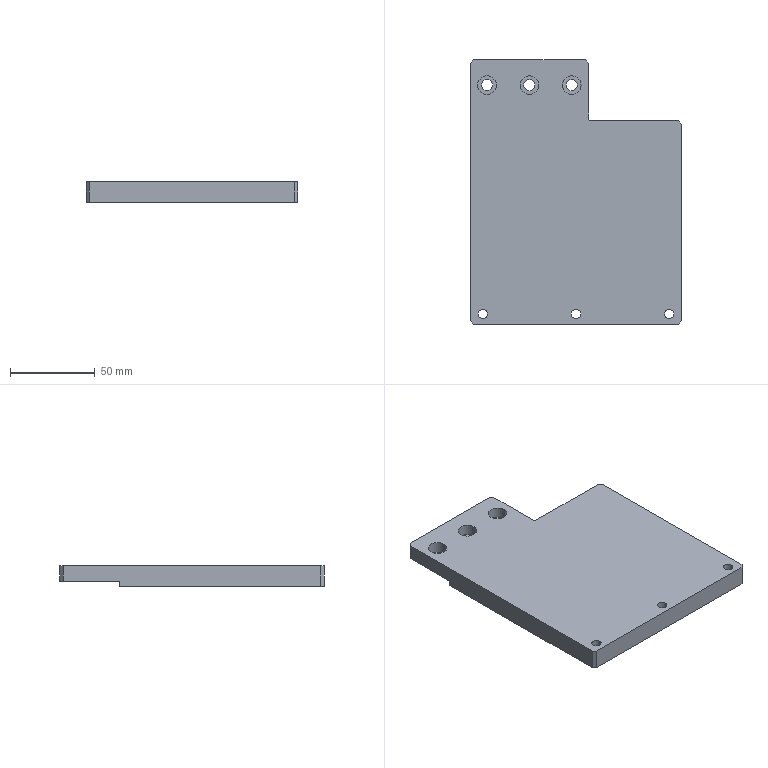Part | SolidWorks | features HoleWzd 2, ICE 2, Chamfer 1, Extrusion 1, Fillet 1 | 1 solid | 46 faces | box 125 x 156 x 12 mm | volume 198828 mm3 | cylinder 25 | plane 21 | commonest cylinder face diameters 5.5 x6 6.6 x6 10 x6 11 x6 2 x1
STEP:
#1=CARTESIAN_POINT('',(-8.,63.,5.2));
#2=VERTEX_POINT('',#1);
#3=CARTESIAN_POINT('',(3.,63.,5.2));
#4=VERTEX_POINT('',#3);
#5=CARTESIAN_POINT('',(-2.5,63.,5.2));
#6=DIRECTION('',(0.,0.,1.));
#7=DIRECTION('',(1.,0.,0.));
#8=AXIS2_PLACEMENT_3D('',#5,#6,#7);
#9=CIRCLE('',#8,5.5);
#10=EDGE_CURVE('',#2,#4,#9,.T.);
#11=ORIENTED_EDGE('',*,*,#10,.F.);
#12=CARTESIAN_POINT('',(-8.,63.,12.));
#13=VERTEX_POINT('',#12);
#14=CARTESIAN_POINT('',(-8.,63.,12.));
#15=DIRECTION('',(0.,0.,1.));
#16=VECTOR('',#15,1000.);
#17=LINE('',#14,#16);
#18=EDGE_CURVE('',#2,#13,#17,.T.);
#19=ORIENTED_EDGE('',*,*,#18,.T.);
#20=CARTESIAN_POINT('',(3.,63.,12.));
#21=VERTEX_POINT('',#20);
#22=CARTESIAN_POINT('',(-2.5,63.,12.));
#23=DIRECTION('',(0.,0.,1.));
#24=DIRECTION('',(1.,0.,0.));
#25=AXIS2_PLACEMENT_3D('',#22,#23,#24);
#26=CIRCLE('',#25,5.5);
#27=EDGE_CURVE('',#13,#21,#26,.T.);
#28=ORIENTED_EDGE('',*,*,#27,.T.);
#29=CARTESIAN_POINT('',(3.,63.,12.));
#30=DIRECTION('',(0.,0.,1.));
#31=VECTOR('',#30,1000.);
#32=LINE('',#29,#31);
#33=EDGE_CURVE('',#4,#21,#32,.T.);
#34=ORIENTED_EDGE('',*,*,#33,.F.);
#35=EDGE_LOOP('',(#11,#19,#28,#34));
#36=FACE_OUTER_BOUND('',#35,.T.);
#37=CARTESIAN_POINT('',(-2.5,63.,12.));
#38=DIRECTION('',(0.,0.,1.));
#39=DIRECTION('',(1.,0.,0.));
#40=AXIS2_PLACEMENT_3D('',#37,#38,#39);
#41=CYLINDRICAL_SURFACE('',#40,5.5);
#42=ADVANCED_FACE('',(#36),#41,.F.);
#43=CARTESIAN_POINT('',(-5.8,63.,3.));
#44=VERTEX_POINT('',#43);
#45=CARTESIAN_POINT('',(0.8,63.,3.));
#46=VERTEX_POINT('',#45);
#47=CARTESIAN_POINT('',(-2.5,63.,3.));
#48=DIRECTION('',(0.,0.,1.));
#49=DIRECTION('',(1.,0.,0.));
#50=AXIS2_PLACEMENT_3D('',#47,#48,#49);
#51=CIRCLE('',#50,3.3);
#52=EDGE_CURVE('',#44,#46,#51,.T.);
#53=ORIENTED_EDGE('',*,*,#52,.F.);
#54=CARTESIAN_POINT('',(-5.8,63.,5.2));
#55=VERTEX_POINT('',#54);
#56=CARTESIAN_POINT('',(-5.8,63.,12.));
#57=DIRECTION('',(0.,0.,1.));
#58=VECTOR('',#57,1000.);
#59=LINE('',#56,#58);
#60=EDGE_CURVE('',#44,#55,#59,.T.);
#61=ORIENTED_EDGE('',*,*,#60,.T.);
#62=CARTESIAN_POINT('',(0.8,63.,5.2));
#63=VERTEX_POINT('',#62);
#64=CARTESIAN_POINT('',(-2.5,63.,5.2));
#65=DIRECTION('',(0.,0.,1.));
#66=DIRECTION('',(1.,0.,0.));
#67=AXIS2_PLACEMENT_3D('',#64,#65,#66);
#68=CIRCLE('',#67,3.3);
#69=EDGE_CURVE('',#55,#63,#68,.T.);
#70=ORIENTED_EDGE('',*,*,#69,.T.);
#71=CARTESIAN_POINT('',(0.8,63.,12.));
#72=DIRECTION('',(0.,0.,1.));
#73=VECTOR('',#72,1000.);
#74=LINE('',#71,#73);
#75=EDGE_CURVE('',#46,#63,#74,.T.);
#76=ORIENTED_EDGE('',*,*,#75,.F.);
#77=EDGE_LOOP('',(#53,#61,#70,#76));
#78=FACE_OUTER_BOUND('',#77,.T.);
#79=CARTESIAN_POINT('',(-2.5,63.,12.));
#80=DIRECTION('',(0.,0.,1.));
#81=DIRECTION('',(1.,0.,0.));
#82=AXIS2_PLACEMENT_3D('',#79,#80,#81);
#83=CYLINDRICAL_SURFACE('',#82,3.3);
#84=ADVANCED_FACE('',(#78),#83,.F.);
#85=CARTESIAN_POINT('',(-33.,63.,5.2));
#86=VERTEX_POINT('',#85);
#87=CARTESIAN_POINT('',(-22.,63.,5.2));
#88=VERTEX_POINT('',#87);
#89=CARTESIAN_POINT('',(-27.5,63.,5.2));
#90=DIRECTION('',(0.,0.,1.));
#91=DIRECTION('',(1.,0.,0.));
#92=AXIS2_PLACEMENT_3D('',#89,#90,#91);
#93=CIRCLE('',#92,5.5);
#94=EDGE_CURVE('',#86,#88,#93,.T.);
#95=ORIENTED_EDGE('',*,*,#94,.F.);
#96=CARTESIAN_POINT('',(-33.,63.,12.));
#97=VERTEX_POINT('',#96);
#98=CARTESIAN_POINT('',(-33.,63.,12.));
#99=DIRECTION('',(0.,0.,1.));
#100=VECTOR('',#99,1000.);
#101=LINE('',#98,#100);
#102=EDGE_CURVE('',#86,#97,#101,.T.);
#103=ORIENTED_EDGE('',*,*,#102,.T.);
#104=CARTESIAN_POINT('',(-22.,63.,12.));
#105=VERTEX_POINT('',#104);
#106=CARTESIAN_POINT('',(-27.5,63.,12.));
#107=DIRECTION('',(0.,0.,1.));
#108=DIRECTION('',(1.,0.,0.));
#109=AXIS2_PLACEMENT_3D('',#106,#107,#108);
#110=CIRCLE('',#109,5.5);
#111=EDGE_CURVE('',#97,#105,#110,.T.);
#112=ORIENTED_EDGE('',*,*,#111,.T.);
#113=CARTESIAN_POINT('',(-22.,63.,12.));
#114=DIRECTION('',(0.,0.,1.));
#115=VECTOR('',#114,1000.);
#116=LINE('',#113,#115);
#117=EDGE_CURVE('',#88,#105,#116,.T.);
#118=ORIENTED_EDGE('',*,*,#117,.F.);
#119=EDGE_LOOP('',(#95,#103,#112,#118));
#120=FACE_OUTER_BOUND('',#119,.T.);
#121=CARTESIAN_POINT('',(-27.5,63.,12.));
#122=DIRECTION('',(0.,0.,1.));
#123=DIRECTION('',(1.,0.,0.));
#124=AXIS2_PLACEMENT_3D('',#121,#122,#123);
#125=CYLINDRICAL_SURFACE('',#124,5.5);
#126=ADVANCED_FACE('',(#120),#125,.F.);
#127=CARTESIAN_POINT('',(-30.8,63.,3.));
#128=VERTEX_POINT('',#127);
#129=CARTESIAN_POINT('',(-24.2,63.,3.));
#130=VERTEX_POINT('',#129);
#131=CARTESIAN_POINT('',(-27.5,63.,3.));
#132=DIRECTION('',(0.,0.,1.));
#133=DIRECTION('',(1.,0.,0.));
#134=AXIS2_PLACEMENT_3D('',#131,#132,#133);
#135=CIRCLE('',#134,3.3);
#136=EDGE_CURVE('',#128,#130,#135,.T.);
#137=ORIENTED_EDGE('',*,*,#136,.F.);
#138=CARTESIAN_POINT('',(-30.8,63.,5.2));
#139=VERTEX_POINT('',#138);
#140=CARTESIAN_POINT('',(-30.8,63.,12.));
#141=DIRECTION('',(0.,0.,1.));
#142=VECTOR('',#141,1000.);
#143=LINE('',#140,#142);
#144=EDGE_CURVE('',#128,#139,#143,.T.);
#145=ORIENTED_EDGE('',*,*,#144,.T.);
#146=CARTESIAN_POINT('',(-24.2,63.,5.2));
#147=VERTEX_POINT('',#146);
#148=CARTESIAN_POINT('',(-27.5,63.,5.2));
#149=DIRECTION('',(0.,0.,1.));
#150=DIRECTION('',(1.,0.,0.));
#151=AXIS2_PLACEMENT_3D('',#148,#149,#150);
#152=CIRCLE('',#151,3.3);
#153=EDGE_CURVE('',#139,#147,#152,.T.);
#154=ORIENTED_EDGE('',*,*,#153,.T.);
#155=CARTESIAN_POINT('',(-24.2,63.,12.));
#156=DIRECTION('',(0.,0.,1.));
#157=VECTOR('',#156,1000.);
#158=LINE('',#155,#157);
#159=EDGE_CURVE('',#130,#147,#158,.T.);
#160=ORIENTED_EDGE('',*,*,#159,.F.);
#161=EDGE_LOOP('',(#137,#145,#154,#160));
#162=FACE_OUTER_BOUND('',#161,.T.);
#163=CARTESIAN_POINT('',(-27.5,63.,12.));
#164=DIRECTION('',(0.,0.,1.));
#165=DIRECTION('',(1.,0.,0.));
#166=AXIS2_PLACEMENT_3D('',#163,#164,#165);
#167=CYLINDRICAL_SURFACE('',#166,3.3);
#168=ADVANCED_FACE('',(#162),#167,.F.);
#169=CARTESIAN_POINT('',(-58.,63.,5.2));
#170=VERTEX_POINT('',#169);
#171=CARTESIAN_POINT('',(-47.,63.,5.2));
#172=VERTEX_POINT('',#171);
#173=CARTESIAN_POINT('',(-52.5,63.,5.2));
#174=DIRECTION('',(0.,0.,1.));
#175=DIRECTION('',(1.,0.,0.));
#176=AXIS2_PLACEMENT_3D('',#173,#174,#175);
#177=CIRCLE('',#176,5.5);
#178=EDGE_CURVE('',#170,#172,#177,.T.);
#179=ORIENTED_EDGE('',*,*,#178,.F.);
#180=CARTESIAN_POINT('',(-58.,63.,12.));
#181=VERTEX_POINT('',#180);
#182=CARTESIAN_POINT('',(-58.,63.,12.));
#183=DIRECTION('',(0.,0.,1.));
#184=VECTOR('',#183,1000.);
#185=LINE('',#182,#184);
#186=EDGE_CURVE('',#170,#181,#185,.T.);
#187=ORIENTED_EDGE('',*,*,#186,.T.);
#188=CARTESIAN_POINT('',(-47.,63.,12.));
#189=VERTEX_POINT('',#188);
#190=CARTESIAN_POINT('',(-52.5,63.,12.));
#191=DIRECTION('',(0.,0.,1.));
#192=DIRECTION('',(1.,0.,0.));
#193=AXIS2_PLACEMENT_3D('',#190,#191,#192);
#194=CIRCLE('',#193,5.5);
#195=EDGE_CURVE('',#181,#189,#194,.T.);
#196=ORIENTED_EDGE('',*,*,#195,.T.);
#197=CARTESIAN_POINT('',(-47.,63.,12.));
#198=DIRECTION('',(0.,0.,1.));
#199=VECTOR('',#198,1000.);
#200=LINE('',#197,#199);
#201=EDGE_CURVE('',#172,#189,#200,.T.);
#202=ORIENTED_EDGE('',*,*,#201,.F.);
#203=EDGE_LOOP('',(#179,#187,#196,#202));
#204=FACE_OUTER_BOUND('',#203,.T.);
#205=CARTESIAN_POINT('',(-52.5,63.,12.));
#206=DIRECTION('',(0.,0.,1.));
#207=DIRECTION('',(1.,0.,0.));
#208=AXIS2_PLACEMENT_3D('',#205,#206,#207);
#209=CYLINDRICAL_SURFACE('',#208,5.5);
#210=ADVANCED_FACE('',(#204),#209,.F.);
#211=CARTESIAN_POINT('',(-55.8,63.,3.));
#212=VERTEX_POINT('',#211);
#213=CARTESIAN_POINT('',(-49.2,63.,3.));
#214=VERTEX_POINT('',#213);
#215=CARTESIAN_POINT('',(-52.5,63.,3.));
#216=DIRECTION('',(0.,0.,1.));
#217=DIRECTION('',(1.,0.,0.));
#218=AXIS2_PLACEMENT_3D('',#215,#216,#217);
#219=CIRCLE('',#218,3.3);
#220=EDGE_CURVE('',#212,#214,#219,.T.);
#221=ORIENTED_EDGE('',*,*,#220,.F.);
#222=CARTESIAN_POINT('',(-55.8,63.,5.2));
#223=VERTEX_POINT('',#222);
#224=CARTESIAN_POINT('',(-55.8,63.,12.));
#225=DIRECTION('',(0.,0.,1.));
#226=VECTOR('',#225,1000.);
#227=LINE('',#224,#226);
#228=EDGE_CURVE('',#212,#223,#227,.T.);
#229=ORIENTED_EDGE('',*,*,#228,.T.);
#230=CARTESIAN_POINT('',(-49.2,63.,5.2));
#231=VERTEX_POINT('',#230);
#232=CARTESIAN_POINT('',(-52.5,63.,5.2));
#233=DIRECTION('',(0.,0.,1.));
#234=DIRECTION('',(1.,0.,0.));
#235=AXIS2_PLACEMENT_3D('',#232,#233,#234);
#236=CIRCLE('',#235,3.3);
#237=EDGE_CURVE('',#223,#231,#236,.T.);
#238=ORIENTED_EDGE('',*,*,#237,.T.);
#239=CARTESIAN_POINT('',(-49.2,63.,12.));
#240=DIRECTION('',(0.,0.,1.));
#241=VECTOR('',#240,1000.);
#242=LINE('',#239,#241);
#243=EDGE_CURVE('',#214,#231,#242,.T.);
#244=ORIENTED_EDGE('',*,*,#243,.F.);
#245=EDGE_LOOP('',(#221,#229,#238,#244));
#246=FACE_OUTER_BOUND('',#245,.T.);
#247=CARTESIAN_POINT('',(-52.5,63.,12.));
#248=DIRECTION('',(0.,0.,1.));
#249=DIRECTION('',(1.,0.,0.));
#250=AXIS2_PLACEMENT_3D('',#247,#248,#249);
#251=CYLINDRICAL_SURFACE('',#250,3.3);
#252=ADVANCED_FACE('',(#246),#251,.F.);
#253=CARTESIAN_POINT('',(60.,-72.,5.7));
#254=VERTEX_POINT('',#253);
#255=CARTESIAN_POINT('',(50.,-72.,5.7));
#256=VERTEX_POINT('',#255);
#257=CARTESIAN_POINT('',(55.,-72.,5.7));
#258=DIRECTION('',(0.,0.,-1.));
#259=DIRECTION('',(-1.,0.,0.));
#260=AXIS2_PLACEMENT_3D('',#257,#258,#259);
#261=CIRCLE('',#260,5.);
#262=EDGE_CURVE('',#254,#256,#261,.T.);
#263=ORIENTED_EDGE('',*,*,#262,.F.);
#264=CARTESIAN_POINT('',(60.,-72.,0.));
#265=VERTEX_POINT('',#264);
#266=CARTESIAN_POINT('',(60.,-72.,0.));
#267=DIRECTION('',(0.,0.,-1.));
#268=VECTOR('',#267,1000.);
#269=LINE('',#266,#268);
#270=EDGE_CURVE('',#254,#265,#269,.T.);
#271=ORIENTED_EDGE('',*,*,#270,.T.);
#272=CARTESIAN_POINT('',(50.,-72.,0.));
#273=VERTEX_POINT('',#272);
#274=CARTESIAN_POINT('',(55.,-72.,0.));
#275=DIRECTION('',(0.,0.,-1.));
#276=DIRECTION('',(-1.,0.,0.));
#277=AXIS2_PLACEMENT_3D('',#274,#275,#276);
#278=CIRCLE('',#277,5.);
#279=EDGE_CURVE('',#265,#273,#278,.T.);
#280=ORIENTED_EDGE('',*,*,#279,.T.);
#281=CARTESIAN_POINT('',(50.,-72.,0.));
#282=DIRECTION('',(0.,0.,-1.));
#283=VECTOR('',#282,1000.);
#284=LINE('',#281,#283);
#285=EDGE_CURVE('',#256,#273,#284,.T.);
#286=ORIENTED_EDGE('',*,*,#285,.F.);
#287=EDGE_LOOP('',(#263,#271,#280,#286));
#288=FACE_OUTER_BOUND('',#287,.T.);
#289=CARTESIAN_POINT('',(55.,-72.,0.));
#290=DIRECTION('',(0.,0.,-1.));
#291=DIRECTION('',(-1.,0.,0.));
#292=AXIS2_PLACEMENT_3D('',#289,#290,#291);
#293=CYLINDRICAL_SURFACE('',#292,5.);
#294=ADVANCED_FACE('',(#288),#293,.F.);
#295=CARTESIAN_POINT('',(57.75,-72.,12.));
#296=VERTEX_POINT('',#295);
#297=CARTESIAN_POINT('',(52.25,-72.,12.));
#298=VERTEX_POINT('',#297);
#299=CARTESIAN_POINT('',(55.,-72.,12.));
#300=DIRECTION('',(0.,0.,-1.));
#301=DIRECTION('',(-1.,0.,0.));
#302=AXIS2_PLACEMENT_3D('',#299,#300,#301);
#303=CIRCLE('',#302,2.75);
#304=EDGE_CURVE('',#296,#298,#303,.T.);
#305=ORIENTED_EDGE('',*,*,#304,.F.);
#306=CARTESIAN_POINT('',(57.75,-72.,5.7));
#307=VERTEX_POINT('',#306);
#308=CARTESIAN_POINT('',(57.75,-72.,0.));
#309=DIRECTION('',(0.,0.,-1.));
#310=VECTOR('',#309,1000.);
#311=LINE('',#308,#310);
#312=EDGE_CURVE('',#296,#307,#311,.T.);
#313=ORIENTED_EDGE('',*,*,#312,.T.);
#314=CARTESIAN_POINT('',(52.25,-72.,5.7));
#315=VERTEX_POINT('',#314);
#316=CARTESIAN_POINT('',(55.,-72.,5.7));
#317=DIRECTION('',(0.,0.,-1.));
#318=DIRECTION('',(-1.,0.,0.));
#319=AXIS2_PLACEMENT_3D('',#316,#317,#318);
#320=CIRCLE('',#319,2.75);
#321=EDGE_CURVE('',#307,#315,#320,.T.);
#322=ORIENTED_EDGE('',*,*,#321,.T.);
#323=CARTESIAN_POINT('',(52.25,-72.,0.));
#324=DIRECTION('',(0.,0.,-1.));
#325=VECTOR('',#324,1000.);
#326=LINE('',#323,#325);
#327=EDGE_CURVE('',#298,#315,#326,.T.);
#328=ORIENTED_EDGE('',*,*,#327,.F.);
#329=EDGE_LOOP('',(#305,#313,#322,#328));
#330=FACE_OUTER_BOUND('',#329,.T.);
#331=CARTESIAN_POINT('',(55.,-72.,0.));
#332=DIRECTION('',(0.,0.,-1.));
#333=DIRECTION('',(-1.,0.,0.));
#334=AXIS2_PLACEMENT_3D('',#331,#332,#333);
#335=CYLINDRICAL_SURFACE('',#334,2.75);
#336=ADVANCED_FACE('',(#330),#335,.F.);
#337=CARTESIAN_POINT('',(5.,-72.,5.7));
#338=VERTEX_POINT('',#337);
#339=CARTESIAN_POINT('',(-5.,-72.,5.7));
#340=VERTEX_POINT('',#339);
#341=CARTESIAN_POINT('',(0.,-72.,5.7));
#342=DIRECTION('',(0.,0.,-1.));
#343=DIRECTION('',(-1.,0.,0.));
#344=AXIS2_PLACEMENT_3D('',#341,#342,#343);
#345=CIRCLE('',#344,5.);
#346=EDGE_CURVE('',#338,#340,#345,.T.);
#347=ORIENTED_EDGE('',*,*,#346,.F.);
#348=CARTESIAN_POINT('',(5.,-72.,0.));
#349=VERTEX_POINT('',#348);
#350=CARTESIAN_POINT('',(5.,-72.,0.));
#351=DIRECTION('',(0.,0.,-1.));
#352=VECTOR('',#351,1000.);
#353=LINE('',#350,#352);
#354=EDGE_CURVE('',#338,#349,#353,.T.);
#355=ORIENTED_EDGE('',*,*,#354,.T.);
#356=CARTESIAN_POINT('',(-5.,-72.,0.));
#357=VERTEX_POINT('',#356);
#358=CARTESIAN_POINT('',(0.,-72.,0.));
#359=DIRECTION('',(0.,0.,-1.));
#360=DIRECTION('',(-1.,0.,0.));
#361=AXIS2_PLACEMENT_3D('',#358,#359,#360);
#362=CIRCLE('',#361,5.);
#363=EDGE_CURVE('',#349,#357,#362,.T.);
#364=ORIENTED_EDGE('',*,*,#363,.T.);
#365=CARTESIAN_POINT('',(-5.,-72.,0.));
#366=DIRECTION('',(0.,0.,-1.));
#367=VECTOR('',#366,1000.);
#368=LINE('',#365,#367);
#369=EDGE_CURVE('',#340,#357,#368,.T.);
#370=ORIENTED_EDGE('',*,*,#369,.F.);
#371=EDGE_LOOP('',(#347,#355,#364,#370));
#372=FACE_OUTER_BOUND('',#371,.T.);
#373=CARTESIAN_POINT('',(0.,-72.,0.));
#374=DIRECTION('',(0.,0.,-1.));
#375=DIRECTION('',(-1.,0.,0.));
#376=AXIS2_PLACEMENT_3D('',#373,#374,#375);
#377=CYLINDRICAL_SURFACE('',#376,5.);
#378=ADVANCED_FACE('',(#372),#377,.F.);
#379=CARTESIAN_POINT('',(2.75,-72.,12.));
#380=VERTEX_POINT('',#379);
#381=CARTESIAN_POINT('',(-2.75,-72.,12.));
#382=VERTEX_POINT('',#381);
#383=CARTESIAN_POINT('',(0.,-72.,12.));
#384=DIRECTION('',(0.,0.,-1.));
#385=DIRECTION('',(-1.,0.,0.));
#386=AXIS2_PLACEMENT_3D('',#383,#384,#385);
#387=CIRCLE('',#386,2.75);
#388=EDGE_CURVE('',#380,#382,#387,.T.);
#389=ORIENTED_EDGE('',*,*,#388,.F.);
#390=CARTESIAN_POINT('',(2.75,-72.,5.7));
#391=VERTEX_POINT('',#390);
#392=CARTESIAN_POINT('',(2.75,-72.,0.));
#393=DIRECTION('',(0.,0.,-1.));
#394=VECTOR('',#393,1000.);
#395=LINE('',#392,#394);
#396=EDGE_CURVE('',#380,#391,#395,.T.);
#397=ORIENTED_EDGE('',*,*,#396,.T.);
#398=CARTESIAN_POINT('',(-2.75,-72.,5.7));
#399=VERTEX_POINT('',#398);
#400=CARTESIAN_POINT('',(0.,-72.,5.7));
#401=DIRECTION('',(0.,0.,-1.));
#402=DIRECTION('',(-1.,0.,0.));
#403=AXIS2_PLACEMENT_3D('',#400,#401,#402);
#404=CIRCLE('',#403,2.75);
#405=EDGE_CURVE('',#391,#399,#404,.T.);
#406=ORIENTED_EDGE('',*,*,#405,.T.);
#407=CARTESIAN_POINT('',(-2.75,-72.,0.));
#408=DIRECTION('',(0.,0.,-1.));
#409=VECTOR('',#408,1000.);
#410=LINE('',#407,#409);
#411=EDGE_CURVE('',#382,#399,#410,.T.);
#412=ORIENTED_EDGE('',*,*,#411,.F.);
#413=EDGE_LOOP('',(#389,#397,#406,#412));
#414=FACE_OUTER_BOUND('',#413,.T.);
#415=CARTESIAN_POINT('',(0.,-72.,0.));
#416=DIRECTION('',(0.,0.,-1.));
#417=DIRECTION('',(-1.,0.,0.));
#418=AXIS2_PLACEMENT_3D('',#415,#416,#417);
#419=CYLINDRICAL_SURFACE('',#418,2.75);
#420=ADVANCED_FACE('',(#414),#419,.F.);
#421=CARTESIAN_POINT('',(-50.,-72.,5.7));
#422=VERTEX_POINT('',#421);
#423=CARTESIAN_POINT('',(-60.,-72.,5.7));
#424=VERTEX_POINT('',#423);
#425=CARTESIAN_POINT('',(-55.,-72.,5.7));
#426=DIRECTION('',(0.,0.,-1.));
#427=DIRECTION('',(-1.,0.,0.));
#428=AXIS2_PLACEMENT_3D('',#425,#426,#427);
#429=CIRCLE('',#428,5.);
#430=EDGE_CURVE('',#422,#424,#429,.T.);
#431=ORIENTED_EDGE('',*,*,#430,.F.);
#432=CARTESIAN_POINT('',(-50.,-72.,0.));
#433=VERTEX_POINT('',#432);
#434=CARTESIAN_POINT('',(-50.,-72.,0.));
#435=DIRECTION('',(0.,0.,-1.));
#436=VECTOR('',#435,1000.);
#437=LINE('',#434,#436);
#438=EDGE_CURVE('',#422,#433,#437,.T.);
#439=ORIENTED_EDGE('',*,*,#438,.T.);
#440=CARTESIAN_POINT('',(-60.,-72.,0.));
#441=VERTEX_POINT('',#440);
#442=CARTESIAN_POINT('',(-55.,-72.,0.));
#443=DIRECTION('',(0.,0.,-1.));
#444=DIRECTION('',(-1.,0.,0.));
#445=AXIS2_PLACEMENT_3D('',#442,#443,#444);
#446=CIRCLE('',#445,5.);
#447=EDGE_CURVE('',#433,#441,#446,.T.);
#448=ORIENTED_EDGE('',*,*,#447,.T.);
#449=CARTESIAN_POINT('',(-60.,-72.,0.));
#450=DIRECTION('',(0.,0.,-1.));
#451=VECTOR('',#450,1000.);
#452=LINE('',#449,#451);
#453=EDGE_CURVE('',#424,#441,#452,.T.);
#454=ORIENTED_EDGE('',*,*,#453,.F.);
#455=EDGE_LOOP('',(#431,#439,#448,#454));
#456=FACE_OUTER_BOUND('',#455,.T.);
#457=CARTESIAN_POINT('',(-55.,-72.,0.));
#458=DIRECTION('',(0.,0.,-1.));
#459=DIRECTION('',(-1.,0.,0.));
#460=AXIS2_PLACEMENT_3D('',#457,#458,#459);
#461=CYLINDRICAL_SURFACE('',#460,5.);
#462=ADVANCED_FACE('',(#456),#461,.F.);
#463=CARTESIAN_POINT('',(-52.25,-72.,12.));
#464=VERTEX_POINT('',#463);
#465=CARTESIAN_POINT('',(-57.75,-72.,12.));
#466=VERTEX_POINT('',#465);
#467=CARTESIAN_POINT('',(-55.,-72.,12.));
#468=DIRECTION('',(0.,0.,-1.));
#469=DIRECTION('',(-1.,0.,0.));
#470=AXIS2_PLACEMENT_3D('',#467,#468,#469);
#471=CIRCLE('',#470,2.75);
#472=EDGE_CURVE('',#464,#466,#471,.T.);
#473=ORIENTED_EDGE('',*,*,#472,.F.);
#474=CARTESIAN_POINT('',(-52.25,-72.,5.7));
#475=VERTEX_POINT('',#474);
#476=CARTESIAN_POINT('',(-52.25,-72.,0.));
#477=DIRECTION('',(0.,0.,-1.));
#478=VECTOR('',#477,1000.);
#479=LINE('',#476,#478);
#480=EDGE_CURVE('',#464,#475,#479,.T.);
#481=ORIENTED_EDGE('',*,*,#480,.T.);
#482=CARTESIAN_POINT('',(-57.75,-72.,5.7));
#483=VERTEX_POINT('',#482);
#484=CARTESIAN_POINT('',(-55.,-72.,5.7));
#485=DIRECTION('',(0.,0.,-1.));
#486=DIRECTION('',(-1.,0.,0.));
#487=AXIS2_PLACEMENT_3D('',#484,#485,#486);
#488=CIRCLE('',#487,2.75);
#489=EDGE_CURVE('',#475,#483,#488,.T.);
#490=ORIENTED_EDGE('',*,*,#489,.T.);
#491=CARTESIAN_POINT('',(-57.75,-72.,0.));
#492=DIRECTION('',(0.,0.,-1.));
#493=VECTOR('',#492,1000.);
#494=LINE('',#491,#493);
#495=EDGE_CURVE('',#466,#483,#494,.T.);
#496=ORIENTED_EDGE('',*,*,#495,.F.);
#497=EDGE_LOOP('',(#473,#481,#490,#496));
#498=FACE_OUTER_BOUND('',#497,.T.);
#499=CARTESIAN_POINT('',(-55.,-72.,0.));
#500=DIRECTION('',(0.,0.,-1.));
#501=DIRECTION('',(-1.,0.,0.));
#502=AXIS2_PLACEMENT_3D('',#499,#500,#501);
#503=CYLINDRICAL_SURFACE('',#502,2.75);
#504=ADVANCED_FACE('',(#498),#503,.F.);
#505=CARTESIAN_POINT('',(62.5,-76.,0.));
#506=VERTEX_POINT('',#505);
#507=CARTESIAN_POINT('',(62.5,40.,0.));
#508=VERTEX_POINT('',#507);
#509=CARTESIAN_POINT('',(62.5,-78.,0.));
#510=DIRECTION('',(0.,1.,0.));
#511=VECTOR('',#510,1000.);
#512=LINE('',#509,#511);
#513=EDGE_CURVE('',#506,#508,#512,.T.);
#514=ORIENTED_EDGE('',*,*,#513,.T.);
#515=CARTESIAN_POINT('',(62.5,40.,12.));
#516=VERTEX_POINT('',#515);
#517=CARTESIAN_POINT('',(62.5,40.,12.));
#518=DIRECTION('',(0.,0.,1.));
#519=VECTOR('',#518,1000.);
#520=LINE('',#517,#519);
#521=EDGE_CURVE('',#508,#516,#520,.T.);
#522=ORIENTED_EDGE('',*,*,#521,.T.);
#523=CARTESIAN_POINT('',(62.5,-76.,12.));
#524=VERTEX_POINT('',#523);
#525=CARTESIAN_POINT('',(62.5,-78.,12.));
#526=DIRECTION('',(0.,1.,0.));
#527=VECTOR('',#526,1000.);
#528=LINE('',#525,#527);
#529=EDGE_CURVE('',#524,#516,#528,.T.);
#530=ORIENTED_EDGE('',*,*,#529,.F.);
#531=CARTESIAN_POINT('',(62.5,-76.,12.));
#532=DIRECTION('',(0.,0.,-1.));
#533=VECTOR('',#532,1000.);
#534=LINE('',#531,#533);
#535=EDGE_CURVE('',#524,#506,#534,.T.);
#536=ORIENTED_EDGE('',*,*,#535,.T.);
#537=EDGE_LOOP('',(#514,#522,#530,#536));
#538=FACE_OUTER_BOUND('',#537,.T.);
#539=CARTESIAN_POINT('',(62.5,-78.,12.));
#540=DIRECTION('',(-1.,0.,0.));
#541=DIRECTION('',(0.,0.,1.));
#542=AXIS2_PLACEMENT_3D('',#539,#540,#541);
#543=PLANE('',#542);
#544=ADVANCED_FACE('',(#538),#543,.F.);
#545=CARTESIAN_POINT('',(5.5,78.,12.));
#546=VERTEX_POINT('',#545);
#547=CARTESIAN_POINT('',(-60.5,78.,12.));
#548=VERTEX_POINT('',#547);
#549=CARTESIAN_POINT('',(-62.5,78.,12.));
#550=DIRECTION('',(-1.,0.,0.));
#551=VECTOR('',#550,1000.);
#552=LINE('',#549,#551);
#553=EDGE_CURVE('',#546,#548,#552,.T.);
#554=ORIENTED_EDGE('',*,*,#553,.F.);
#555=CARTESIAN_POINT('',(5.5,78.,3.));
#556=VERTEX_POINT('',#555);
#557=CARTESIAN_POINT('',(5.5,78.,12.));
#558=DIRECTION('',(0.,0.,-1.));
#559=VECTOR('',#558,1000.);
#560=LINE('',#557,#559);
#561=EDGE_CURVE('',#546,#556,#560,.T.);
#562=ORIENTED_EDGE('',*,*,#561,.T.);
#563=CARTESIAN_POINT('',(-60.5,78.,3.));
#564=VERTEX_POINT('',#563);
#565=CARTESIAN_POINT('',(-62.5,78.,3.));
#566=DIRECTION('',(1.,0.,0.));
#567=VECTOR('',#566,1000.);
#568=LINE('',#565,#567);
#569=EDGE_CURVE('',#564,#556,#568,.T.);
#570=ORIENTED_EDGE('',*,*,#569,.F.);
#571=CARTESIAN_POINT('',(-60.5,78.,12.));
#572=DIRECTION('',(0.,0.,1.));
#573=VECTOR('',#572,1000.);
#574=LINE('',#571,#573);
#575=EDGE_CURVE('',#564,#548,#574,.T.);
#576=ORIENTED_EDGE('',*,*,#575,.T.);
#577=EDGE_LOOP('',(#554,#562,#570,#576));
#578=FACE_OUTER_BOUND('',#577,.T.);
#579=CARTESIAN_POINT('',(-62.5,78.,12.));
#580=DIRECTION('',(0.,-1.,0.));
#581=DIRECTION('',(0.,0.,-1.));
#582=AXIS2_PLACEMENT_3D('',#579,#580,#581);
#583=PLANE('',#582);
#584=ADVANCED_FACE('',(#578),#583,.F.);
#585=CARTESIAN_POINT('',(-62.5,76.,12.));
#586=VERTEX_POINT('',#585);
#587=CARTESIAN_POINT('',(-62.5,-76.,12.));
#588=VERTEX_POINT('',#587);
#589=CARTESIAN_POINT('',(-62.5,-78.,12.));
#590=DIRECTION('',(0.,-1.,0.));
#591=VECTOR('',#590,1000.);
#592=LINE('',#589,#591);
#593=EDGE_CURVE('',#586,#588,#592,.T.);
#594=ORIENTED_EDGE('',*,*,#593,.F.);
#595=CARTESIAN_POINT('',(-62.5,76.,3.));
#596=VERTEX_POINT('',#595);
#597=CARTESIAN_POINT('',(-62.5,76.,12.));
#598=DIRECTION('',(0.,0.,-1.));
#599=VECTOR('',#598,1000.);
#600=LINE('',#597,#599);
#601=EDGE_CURVE('',#586,#596,#600,.T.);
#602=ORIENTED_EDGE('',*,*,#601,.T.);
#603=CARTESIAN_POINT('',(-62.5,43.,3.));
#604=VERTEX_POINT('',#603);
#605=CARTESIAN_POINT('',(-62.5,78.,3.));
#606=DIRECTION('',(0.,1.,0.));
#607=VECTOR('',#606,1000.);
#608=LINE('',#605,#607);
#609=EDGE_CURVE('',#604,#596,#608,.T.);
#610=ORIENTED_EDGE('',*,*,#609,.F.);
#611=CARTESIAN_POINT('',(-62.5,43.,0.));
#612=VERTEX_POINT('',#611);
#613=CARTESIAN_POINT('',(-62.5,43.,3.));
#614=DIRECTION('',(0.,0.,-1.));
#615=VECTOR('',#614,1000.);
#616=LINE('',#613,#615);
#617=EDGE_CURVE('',#604,#612,#616,.T.);
#618=ORIENTED_EDGE('',*,*,#617,.T.);
#619=CARTESIAN_POINT('',(-62.5,-76.,0.));
#620=VERTEX_POINT('',#619);
#621=CARTESIAN_POINT('',(-62.5,-78.,0.));
#622=DIRECTION('',(0.,-1.,0.));
#623=VECTOR('',#622,1000.);
#624=LINE('',#621,#623);
#625=EDGE_CURVE('',#612,#620,#624,.T.);
#626=ORIENTED_EDGE('',*,*,#625,.T.);
#627=CARTESIAN_POINT('',(-62.5,-76.,12.));
#628=DIRECTION('',(0.,0.,1.));
#629=VECTOR('',#628,1000.);
#630=LINE('',#627,#629);
#631=EDGE_CURVE('',#620,#588,#630,.T.);
#632=ORIENTED_EDGE('',*,*,#631,.T.);
#633=EDGE_LOOP('',(#594,#602,#610,#618,#626,#632));
#634=FACE_OUTER_BOUND('',#633,.T.);
#635=CARTESIAN_POINT('',(-62.5,-78.,12.));
#636=DIRECTION('',(1.,0.,0.));
#637=DIRECTION('',(0.,0.,-1.));
#638=AXIS2_PLACEMENT_3D('',#635,#636,#637);
#639=PLANE('',#638);
#640=ADVANCED_FACE('',(#634),#639,.F.);
#641=CARTESIAN_POINT('',(-60.5,-78.,0.));
#642=VERTEX_POINT('',#641);
#643=CARTESIAN_POINT('',(60.5,-78.,0.));
#644=VERTEX_POINT('',#643);
#645=CARTESIAN_POINT('',(-62.5,-78.,0.));
#646=DIRECTION('',(1.,0.,0.));
#647=VECTOR('',#646,1000.);
#648=LINE('',#645,#647);
#649=EDGE_CURVE('',#642,#644,#648,.T.);
#650=ORIENTED_EDGE('',*,*,#649,.T.);
#651=CARTESIAN_POINT('',(60.5,-78.,12.));
#652=VERTEX_POINT('',#651);
#653=CARTESIAN_POINT('',(60.5,-78.,12.));
#654=DIRECTION('',(0.,0.,1.));
#655=VECTOR('',#654,1000.);
#656=LINE('',#653,#655);
#657=EDGE_CURVE('',#644,#652,#656,.T.);
#658=ORIENTED_EDGE('',*,*,#657,.T.);
#659=CARTESIAN_POINT('',(-60.5,-78.,12.));
#660=VERTEX_POINT('',#659);
#661=CARTESIAN_POINT('',(-62.5,-78.,12.));
#662=DIRECTION('',(1.,0.,0.));
#663=VECTOR('',#662,1000.);
#664=LINE('',#661,#663);
#665=EDGE_CURVE('',#660,#652,#664,.T.);
#666=ORIENTED_EDGE('',*,*,#665,.F.);
#667=CARTESIAN_POINT('',(-60.5,-78.,12.));
#668=DIRECTION('',(0.,0.,-1.));
#669=VECTOR('',#668,1000.);
#670=LINE('',#667,#669);
#671=EDGE_CURVE('',#660,#642,#670,.T.);
#672=ORIENTED_EDGE('',*,*,#671,.T.);
#673=EDGE_LOOP('',(#650,#658,#666,#672));
#674=FACE_OUTER_BOUND('',#673,.T.);
#675=CARTESIAN_POINT('',(-62.5,-78.,12.));
#676=DIRECTION('',(0.,1.,0.));
#677=DIRECTION('',(0.,0.,1.));
#678=AXIS2_PLACEMENT_3D('',#675,#676,#677);
#679=PLANE('',#678);
#680=ADVANCED_FACE('',(#674),#679,.F.);
#681=CARTESIAN_POINT('',(-2.5,63.,12.));
#682=DIRECTION('',(0.,0.,1.));
#683=DIRECTION('',(1.,0.,0.));
#684=AXIS2_PLACEMENT_3D('',#681,#682,#683);
#685=CIRCLE('',#684,5.5);
#686=EDGE_CURVE('',#21,#13,#685,.T.);
#687=ORIENTED_EDGE('',*,*,#686,.F.);
#688=ORIENTED_EDGE('',*,*,#27,.F.);
#689=EDGE_LOOP('',(#687,#688));
#690=FACE_BOUND('',#689,.T.);
#691=CARTESIAN_POINT('',(-27.5,63.,12.));
#692=DIRECTION('',(0.,0.,1.));
#693=DIRECTION('',(1.,0.,0.));
#694=AXIS2_PLACEMENT_3D('',#691,#692,#693);
#695=CIRCLE('',#694,5.5);
#696=EDGE_CURVE('',#105,#97,#695,.T.);
#697=ORIENTED_EDGE('',*,*,#696,.F.);
#698=ORIENTED_EDGE('',*,*,#111,.F.);
#699=EDGE_LOOP('',(#697,#698));
#700=FACE_BOUND('',#699,.T.);
#701=CARTESIAN_POINT('',(-52.5,63.,12.));
#702=DIRECTION('',(0.,0.,1.));
#703=DIRECTION('',(1.,0.,0.));
#704=AXIS2_PLACEMENT_3D('',#701,#702,#703);
#705=CIRCLE('',#704,5.5);
#706=EDGE_CURVE('',#189,#181,#705,.T.);
#707=ORIENTED_EDGE('',*,*,#706,.F.);
#708=ORIENTED_EDGE('',*,*,#195,.F.);
#709=EDGE_LOOP('',(#707,#708));
#710=FACE_BOUND('',#709,.T.);
#711=CARTESIAN_POINT('',(55.,-72.,12.));
#712=DIRECTION('',(0.,0.,-1.));
#713=DIRECTION('',(-1.,0.,0.));
#714=AXIS2_PLACEMENT_3D('',#711,#712,#713);
#715=CIRCLE('',#714,2.75);
#716=EDGE_CURVE('',#298,#296,#715,.T.);
#717=ORIENTED_EDGE('',*,*,#716,.T.);
#718=ORIENTED_EDGE('',*,*,#304,.T.);
#719=EDGE_LOOP('',(#717,#718));
#720=FACE_BOUND('',#719,.T.);
#721=CARTESIAN_POINT('',(0.,-72.,12.));
#722=DIRECTION('',(0.,0.,-1.));
#723=DIRECTION('',(-1.,0.,0.));
#724=AXIS2_PLACEMENT_3D('',#721,#722,#723);
#725=CIRCLE('',#724,2.75);
#726=EDGE_CURVE('',#382,#380,#725,.T.);
#727=ORIENTED_EDGE('',*,*,#726,.T.);
#728=ORIENTED_EDGE('',*,*,#388,.T.);
#729=EDGE_LOOP('',(#727,#728));
#730=FACE_BOUND('',#729,.T.);
#731=CARTESIAN_POINT('',(-55.,-72.,12.));
#732=DIRECTION('',(0.,0.,-1.));
#733=DIRECTION('',(-1.,0.,0.));
#734=AXIS2_PLACEMENT_3D('',#731,#732,#733);
#735=CIRCLE('',#734,2.75);
#736=EDGE_CURVE('',#466,#464,#735,.T.);
#737=ORIENTED_EDGE('',*,*,#736,.T.);
#738=ORIENTED_EDGE('',*,*,#472,.T.);
#739=EDGE_LOOP('',(#737,#738));
#740=FACE_BOUND('',#739,.T.);
#741=CARTESIAN_POINT('',(7.5,76.,12.));
#742=VERTEX_POINT('',#741);
#743=CARTESIAN_POINT('',(7.5,43.,12.));
#744=VERTEX_POINT('',#743);
#745=CARTESIAN_POINT('',(7.5,78.,12.));
#746=DIRECTION('',(0.,-1.,0.));
#747=VECTOR('',#746,1000.);
#748=LINE('',#745,#747);
#749=EDGE_CURVE('',#742,#744,#748,.T.);
#750=ORIENTED_EDGE('',*,*,#749,.F.);
#751=CARTESIAN_POINT('',(7.5,76.,12.));
#752=DIRECTION('',(-0.7071,0.7071,0.));
#753=VECTOR('',#752,1000.);
#754=LINE('',#751,#753);
#755=EDGE_CURVE('',#742,#546,#754,.T.);
#756=ORIENTED_EDGE('',*,*,#755,.T.);
#757=ORIENTED_EDGE('',*,*,#553,.T.);
#758=CARTESIAN_POINT('',(-62.5,76.,12.));
#759=DIRECTION('',(-0.7071,-0.7071,0.));
#760=VECTOR('',#759,1000.);
#761=LINE('',#758,#760);
#762=EDGE_CURVE('',#548,#586,#761,.T.);
#763=ORIENTED_EDGE('',*,*,#762,.T.);
#764=ORIENTED_EDGE('',*,*,#593,.T.);
#765=CARTESIAN_POINT('',(-60.5,-78.,12.));
#766=DIRECTION('',(0.7071,-0.7071,0.));
#767=VECTOR('',#766,1000.);
#768=LINE('',#765,#767);
#769=EDGE_CURVE('',#588,#660,#768,.T.);
#770=ORIENTED_EDGE('',*,*,#769,.T.);
#771=ORIENTED_EDGE('',*,*,#665,.T.);
#772=CARTESIAN_POINT('',(62.5,-76.,12.));
#773=DIRECTION('',(0.7071,0.7071,0.));
#774=VECTOR('',#773,1000.);
#775=LINE('',#772,#774);
#776=EDGE_CURVE('',#652,#524,#775,.T.);
#777=ORIENTED_EDGE('',*,*,#776,.T.);
#778=ORIENTED_EDGE('',*,*,#529,.T.);
#779=CARTESIAN_POINT('',(60.5,42.,12.));
#780=VERTEX_POINT('',#779);
#781=CARTESIAN_POINT('',(62.5,40.,12.));
#782=DIRECTION('',(-0.7071,0.7071,0.));
#783=VECTOR('',#782,1000.);
#784=LINE('',#781,#783);
#785=EDGE_CURVE('',#516,#780,#784,.T.);
#786=ORIENTED_EDGE('',*,*,#785,.T.);
#787=CARTESIAN_POINT('',(8.5,42.,12.));
#788=VERTEX_POINT('',#787);
#789=CARTESIAN_POINT('',(62.5,42.,12.));
#790=DIRECTION('',(1.,0.,0.));
#791=VECTOR('',#790,1000.);
#792=LINE('',#789,#791);
#793=EDGE_CURVE('',#788,#780,#792,.T.);
#794=ORIENTED_EDGE('',*,*,#793,.F.);
#795=CARTESIAN_POINT('',(8.5,43.,12.));
#796=DIRECTION('',(0.,0.,-1.));
#797=DIRECTION('',(-1.,0.,0.));
#798=AXIS2_PLACEMENT_3D('',#795,#796,#797);
#799=CIRCLE('',#798,1.);
#800=EDGE_CURVE('',#788,#744,#799,.T.);
#801=ORIENTED_EDGE('',*,*,#800,.T.);
#802=EDGE_LOOP('',(#750,#756,#757,#763,#764,#770,#771,#777,#778,#786,#794,#801));
#803=FACE_OUTER_BOUND('',#802,.T.);
#804=CARTESIAN_POINT('',(0.,0.,12.));
#805=DIRECTION('',(0.,0.,-1.));
#806=DIRECTION('',(-1.,0.,0.));
#807=AXIS2_PLACEMENT_3D('',#804,#805,#806);
#808=PLANE('',#807);
#809=ADVANCED_FACE('',(#690,#700,#710,#720,#730,#740,#803),#808,.F.);
#810=CARTESIAN_POINT('',(55.,-72.,0.));
#811=DIRECTION('',(0.,0.,-1.));
#812=DIRECTION('',(-1.,0.,0.));
#813=AXIS2_PLACEMENT_3D('',#810,#811,#812);
#814=CIRCLE('',#813,5.);
#815=EDGE_CURVE('',#273,#265,#814,.T.);
#816=ORIENTED_EDGE('',*,*,#815,.F.);
#817=ORIENTED_EDGE('',*,*,#279,.F.);
#818=EDGE_LOOP('',(#816,#817));
#819=FACE_BOUND('',#818,.T.);
#820=CARTESIAN_POINT('',(0.,-72.,0.));
#821=DIRECTION('',(0.,0.,-1.));
#822=DIRECTION('',(-1.,0.,0.));
#823=AXIS2_PLACEMENT_3D('',#820,#821,#822);
#824=CIRCLE('',#823,5.);
#825=EDGE_CURVE('',#357,#349,#824,.T.);
#826=ORIENTED_EDGE('',*,*,#825,.F.);
#827=ORIENTED_EDGE('',*,*,#363,.F.);
#828=EDGE_LOOP('',(#826,#827));
#829=FACE_BOUND('',#828,.T.);
#830=CARTESIAN_POINT('',(-55.,-72.,0.));
#831=DIRECTION('',(0.,0.,-1.));
#832=DIRECTION('',(-1.,0.,0.));
#833=AXIS2_PLACEMENT_3D('',#830,#831,#832);
#834=CIRCLE('',#833,5.);
#835=EDGE_CURVE('',#441,#433,#834,.T.);
#836=ORIENTED_EDGE('',*,*,#835,.F.);
#837=ORIENTED_EDGE('',*,*,#447,.F.);
#838=EDGE_LOOP('',(#836,#837));
#839=FACE_BOUND('',#838,.T.);
#840=CARTESIAN_POINT('',(7.5,43.,0.));
#841=VERTEX_POINT('',#840);
#842=CARTESIAN_POINT('',(-62.5,43.,0.));
#843=DIRECTION('',(-1.,0.,0.));
#844=VECTOR('',#843,1000.);
#845=LINE('',#842,#844);
#846=EDGE_CURVE('',#841,#612,#845,.T.);
#847=ORIENTED_EDGE('',*,*,#846,.F.);
#848=CARTESIAN_POINT('',(8.5,42.,0.));
#849=VERTEX_POINT('',#848);
#850=CARTESIAN_POINT('',(8.5,43.,0.));
#851=DIRECTION('',(0.,0.,1.));
#852=DIRECTION('',(-1.,0.,0.));
#853=AXIS2_PLACEMENT_3D('',#850,#851,#852);
#854=CIRCLE('',#853,1.);
#855=EDGE_CURVE('',#841,#849,#854,.T.);
#856=ORIENTED_EDGE('',*,*,#855,.T.);
#857=CARTESIAN_POINT('',(60.5,42.,0.));
#858=VERTEX_POINT('',#857);
#859=CARTESIAN_POINT('',(62.5,42.,0.));
#860=DIRECTION('',(1.,0.,0.));
#861=VECTOR('',#860,1000.);
#862=LINE('',#859,#861);
#863=EDGE_CURVE('',#849,#858,#862,.T.);
#864=ORIENTED_EDGE('',*,*,#863,.T.);
#865=CARTESIAN_POINT('',(51.25,51.25,0.));
#866=DIRECTION('',(0.7071,-0.7071,0.));
#867=VECTOR('',#866,1000.);
#868=LINE('',#865,#867);
#869=EDGE_CURVE('',#858,#508,#868,.T.);
#870=ORIENTED_EDGE('',*,*,#869,.T.);
#871=ORIENTED_EDGE('',*,*,#513,.F.);
#872=CARTESIAN_POINT('',(69.25,-69.25,0.));
#873=DIRECTION('',(-0.7071,-0.7071,0.));
#874=VECTOR('',#873,1000.);
#875=LINE('',#872,#874);
#876=EDGE_CURVE('',#506,#644,#875,.T.);
#877=ORIENTED_EDGE('',*,*,#876,.T.);
#878=ORIENTED_EDGE('',*,*,#649,.F.);
#879=CARTESIAN_POINT('',(-69.25,-69.25,0.));
#880=DIRECTION('',(-0.7071,0.7071,0.));
#881=VECTOR('',#880,1000.);
#882=LINE('',#879,#881);
#883=EDGE_CURVE('',#642,#620,#882,.T.);
#884=ORIENTED_EDGE('',*,*,#883,.T.);
#885=ORIENTED_EDGE('',*,*,#625,.F.);
#886=EDGE_LOOP('',(#847,#856,#864,#870,#871,#877,#878,#884,#885));
#887=FACE_OUTER_BOUND('',#886,.T.);
#888=CARTESIAN_POINT('',(0.,0.,0.));
#889=DIRECTION('',(0.,0.,-1.));
#890=DIRECTION('',(-1.,0.,0.));
#891=AXIS2_PLACEMENT_3D('',#888,#889,#890);
#892=PLANE('',#891);
#893=ADVANCED_FACE('',(#819,#829,#839,#887),#892,.T.);
#894=ORIENTED_EDGE('',*,*,#863,.F.);
#895=CARTESIAN_POINT('',(8.5,42.,12.));
#896=DIRECTION('',(0.,0.,1.));
#897=VECTOR('',#896,1000.);
#898=LINE('',#895,#897);
#899=EDGE_CURVE('',#849,#788,#898,.T.);
#900=ORIENTED_EDGE('',*,*,#899,.T.);
#901=ORIENTED_EDGE('',*,*,#793,.T.);
#902=CARTESIAN_POINT('',(60.5,42.,0.));
#903=DIRECTION('',(0.,0.,-1.));
#904=VECTOR('',#903,1000.);
#905=LINE('',#902,#904);
#906=EDGE_CURVE('',#780,#858,#905,.T.);
#907=ORIENTED_EDGE('',*,*,#906,.T.);
#908=EDGE_LOOP('',(#894,#900,#901,#907));
#909=FACE_OUTER_BOUND('',#908,.T.);
#910=CARTESIAN_POINT('',(62.5,42.,0.));
#911=DIRECTION('',(0.,-1.,0.));
#912=DIRECTION('',(1.,0.,0.));
#913=AXIS2_PLACEMENT_3D('',#910,#911,#912);
#914=PLANE('',#913);
#915=ADVANCED_FACE('',(#909),#914,.F.);
#916=ORIENTED_EDGE('',*,*,#749,.T.);
#917=CARTESIAN_POINT('',(7.5,43.,3.));
#918=VERTEX_POINT('',#917);
#919=CARTESIAN_POINT('',(7.5,43.,0.));
#920=DIRECTION('',(0.,0.,-1.));
#921=VECTOR('',#920,1000.);
#922=LINE('',#919,#921);
#923=EDGE_CURVE('',#744,#918,#922,.T.);
#924=ORIENTED_EDGE('',*,*,#923,.T.);
#925=CARTESIAN_POINT('',(7.5,76.,3.));
#926=VERTEX_POINT('',#925);
#927=CARTESIAN_POINT('',(7.5,78.,3.));
#928=DIRECTION('',(0.,-1.,0.));
#929=VECTOR('',#928,1000.);
#930=LINE('',#927,#929);
#931=EDGE_CURVE('',#926,#918,#930,.T.);
#932=ORIENTED_EDGE('',*,*,#931,.F.);
#933=CARTESIAN_POINT('',(7.5,76.,0.));
#934=DIRECTION('',(0.,0.,1.));
#935=VECTOR('',#934,1000.);
#936=LINE('',#933,#935);
#937=EDGE_CURVE('',#926,#742,#936,.T.);
#938=ORIENTED_EDGE('',*,*,#937,.T.);
#939=EDGE_LOOP('',(#916,#924,#932,#938));
#940=FACE_OUTER_BOUND('',#939,.T.);
#941=CARTESIAN_POINT('',(7.5,78.,0.));
#942=DIRECTION('',(-1.,0.,0.));
#943=DIRECTION('',(0.,-1.,0.));
#944=AXIS2_PLACEMENT_3D('',#941,#942,#943);
#945=PLANE('',#944);
#946=ADVANCED_FACE('',(#940),#945,.F.);
#947=ORIENTED_EDGE('',*,*,#846,.T.);
#948=ORIENTED_EDGE('',*,*,#617,.F.);
#949=CARTESIAN_POINT('',(-62.5,43.,3.));
#950=DIRECTION('',(-1.,0.,0.));
#951=VECTOR('',#950,1000.);
#952=LINE('',#949,#951);
#953=EDGE_CURVE('',#918,#604,#952,.T.);
#954=ORIENTED_EDGE('',*,*,#953,.F.);
#955=CARTESIAN_POINT('',(7.5,43.,3.));
#956=DIRECTION('',(0.,0.,-1.));
#957=VECTOR('',#956,1000.);
#958=LINE('',#955,#957);
#959=EDGE_CURVE('',#918,#841,#958,.T.);
#960=ORIENTED_EDGE('',*,*,#959,.T.);
#961=EDGE_LOOP('',(#947,#948,#954,#960));
#962=FACE_OUTER_BOUND('',#961,.T.);
#963=CARTESIAN_POINT('',(-62.5,43.,3.));
#964=DIRECTION('',(0.,-1.,0.));
#965=DIRECTION('',(1.,0.,0.));
#966=AXIS2_PLACEMENT_3D('',#963,#964,#965);
#967=PLANE('',#966);
#968=ADVANCED_FACE('',(#962),#967,.F.);
#969=CARTESIAN_POINT('',(-2.5,63.,3.));
#970=DIRECTION('',(0.,0.,1.));
#971=DIRECTION('',(1.,0.,0.));
#972=AXIS2_PLACEMENT_3D('',#969,#970,#971);
#973=CIRCLE('',#972,3.3);
#974=EDGE_CURVE('',#46,#44,#973,.T.);
#975=ORIENTED_EDGE('',*,*,#974,.T.);
#976=ORIENTED_EDGE('',*,*,#52,.T.);
#977=EDGE_LOOP('',(#975,#976));
#978=FACE_BOUND('',#977,.T.);
#979=CARTESIAN_POINT('',(-27.5,63.,3.));
#980=DIRECTION('',(0.,0.,1.));
#981=DIRECTION('',(1.,0.,0.));
#982=AXIS2_PLACEMENT_3D('',#979,#980,#981);
#983=CIRCLE('',#982,3.3);
#984=EDGE_CURVE('',#130,#128,#983,.T.);
#985=ORIENTED_EDGE('',*,*,#984,.T.);
#986=ORIENTED_EDGE('',*,*,#136,.T.);
#987=EDGE_LOOP('',(#985,#986));
#988=FACE_BOUND('',#987,.T.);
#989=CARTESIAN_POINT('',(-52.5,63.,3.));
#990=DIRECTION('',(0.,0.,1.));
#991=DIRECTION('',(1.,0.,0.));
#992=AXIS2_PLACEMENT_3D('',#989,#990,#991);
#993=CIRCLE('',#992,3.3);
#994=EDGE_CURVE('',#214,#212,#993,.T.);
#995=ORIENTED_EDGE('',*,*,#994,.T.);
#996=ORIENTED_EDGE('',*,*,#220,.T.);
#997=EDGE_LOOP('',(#995,#996));
#998=FACE_BOUND('',#997,.T.);
#999=ORIENTED_EDGE('',*,*,#569,.T.);
#1000=CARTESIAN_POINT('',(7.5,76.,3.));
#1001=DIRECTION('',(0.7071,-0.7071,0.));
#1002=VECTOR('',#1001,1000.);
#1003=LINE('',#1000,#1002);
#1004=EDGE_CURVE('',#556,#926,#1003,.T.);
#1005=ORIENTED_EDGE('',*,*,#1004,.T.);
#1006=ORIENTED_EDGE('',*,*,#931,.T.);
#1007=ORIENTED_EDGE('',*,*,#953,.T.);
#1008=ORIENTED_EDGE('',*,*,#609,.T.);
#1009=CARTESIAN_POINT('',(-62.5,76.,3.));
#1010=DIRECTION('',(0.7071,0.7071,0.));
#1011=VECTOR('',#1010,1000.);
#1012=LINE('',#1009,#1011);
#1013=EDGE_CURVE('',#596,#564,#1012,.T.);
#1014=ORIENTED_EDGE('',*,*,#1013,.T.);
#1015=EDGE_LOOP('',(#999,#1005,#1006,#1007,#1008,#1014));
#1016=FACE_OUTER_BOUND('',#1015,.T.);
#1017=CARTESIAN_POINT('',(0.,0.,3.));
#1018=DIRECTION('',(0.,0.,1.));
#1019=DIRECTION('',(1.,0.,0.));
#1020=AXIS2_PLACEMENT_3D('',#1017,#1018,#1019);
#1021=PLANE('',#1020);
#1022=ADVANCED_FACE('',(#978,#988,#998,#1016),#1021,.F.);
#1023=ORIENTED_EDGE('',*,*,#480,.F.);
#1024=ORIENTED_EDGE('',*,*,#736,.F.);
#1025=ORIENTED_EDGE('',*,*,#495,.T.);
#1026=CARTESIAN_POINT('',(-55.,-72.,5.7));
#1027=DIRECTION('',(0.,0.,-1.));
#1028=DIRECTION('',(-1.,0.,0.));
#1029=AXIS2_PLACEMENT_3D('',#1026,#1027,#1028);
#1030=CIRCLE('',#1029,2.75);
#1031=EDGE_CURVE('',#483,#475,#1030,.T.);
#1032=ORIENTED_EDGE('',*,*,#1031,.T.);
#1033=EDGE_LOOP('',(#1023,#1024,#1025,#1032));
#1034=FACE_OUTER_BOUND('',#1033,.T.);
#1035=CARTESIAN_POINT('',(-55.,-72.,0.));
#1036=DIRECTION('',(0.,0.,-1.));
#1037=DIRECTION('',(-1.,0.,0.));
#1038=AXIS2_PLACEMENT_3D('',#1035,#1036,#1037);
#1039=CYLINDRICAL_SURFACE('',#1038,2.75);
#1040=ADVANCED_FACE('',(#1034),#1039,.F.);
#1041=ORIENTED_EDGE('',*,*,#1031,.F.);
#1042=ORIENTED_EDGE('',*,*,#489,.F.);
#1043=EDGE_LOOP('',(#1041,#1042));
#1044=FACE_BOUND('',#1043,.T.);
#1045=CARTESIAN_POINT('',(-55.,-72.,5.7));
#1046=DIRECTION('',(0.,0.,-1.));
#1047=DIRECTION('',(-1.,0.,0.));
#1048=AXIS2_PLACEMENT_3D('',#1045,#1046,#1047);
#1049=CIRCLE('',#1048,5.);
#1050=EDGE_CURVE('',#424,#422,#1049,.T.);
#1051=ORIENTED_EDGE('',*,*,#1050,.T.);
#1052=ORIENTED_EDGE('',*,*,#430,.T.);
#1053=EDGE_LOOP('',(#1051,#1052));
#1054=FACE_OUTER_BOUND('',#1053,.T.);
#1055=CARTESIAN_POINT('',(-52.25,-72.,5.7));
#1056=DIRECTION('',(0.,0.,1.));
#1057=DIRECTION('',(1.,0.,0.));
#1058=AXIS2_PLACEMENT_3D('',#1055,#1056,#1057);
#1059=PLANE('',#1058);
#1060=ADVANCED_FACE('',(#1044,#1054),#1059,.F.);
#1061=ORIENTED_EDGE('',*,*,#438,.F.);
#1062=ORIENTED_EDGE('',*,*,#1050,.F.);
#1063=ORIENTED_EDGE('',*,*,#453,.T.);
#1064=ORIENTED_EDGE('',*,*,#835,.T.);
#1065=EDGE_LOOP('',(#1061,#1062,#1063,#1064));
#1066=FACE_OUTER_BOUND('',#1065,.T.);
#1067=CARTESIAN_POINT('',(-55.,-72.,0.));
#1068=DIRECTION('',(0.,0.,-1.));
#1069=DIRECTION('',(-1.,0.,0.));
#1070=AXIS2_PLACEMENT_3D('',#1067,#1068,#1069);
#1071=CYLINDRICAL_SURFACE('',#1070,5.);
#1072=ADVANCED_FACE('',(#1066),#1071,.F.);
#1073=ORIENTED_EDGE('',*,*,#396,.F.);
#1074=ORIENTED_EDGE('',*,*,#726,.F.);
#1075=ORIENTED_EDGE('',*,*,#411,.T.);
#1076=CARTESIAN_POINT('',(0.,-72.,5.7));
#1077=DIRECTION('',(0.,0.,-1.));
#1078=DIRECTION('',(-1.,0.,0.));
#1079=AXIS2_PLACEMENT_3D('',#1076,#1077,#1078);
#1080=CIRCLE('',#1079,2.75);
#1081=EDGE_CURVE('',#399,#391,#1080,.T.);
#1082=ORIENTED_EDGE('',*,*,#1081,.T.);
#1083=EDGE_LOOP('',(#1073,#1074,#1075,#1082));
#1084=FACE_OUTER_BOUND('',#1083,.T.);
#1085=CARTESIAN_POINT('',(0.,-72.,0.));
#1086=DIRECTION('',(0.,0.,-1.));
#1087=DIRECTION('',(-1.,0.,0.));
#1088=AXIS2_PLACEMENT_3D('',#1085,#1086,#1087);
#1089=CYLINDRICAL_SURFACE('',#1088,2.75);
#1090=ADVANCED_FACE('',(#1084),#1089,.F.);
#1091=ORIENTED_EDGE('',*,*,#1081,.F.);
#1092=ORIENTED_EDGE('',*,*,#405,.F.);
#1093=EDGE_LOOP('',(#1091,#1092));
#1094=FACE_BOUND('',#1093,.T.);
#1095=CARTESIAN_POINT('',(0.,-72.,5.7));
#1096=DIRECTION('',(0.,0.,-1.));
#1097=DIRECTION('',(-1.,0.,0.));
#1098=AXIS2_PLACEMENT_3D('',#1095,#1096,#1097);
#1099=CIRCLE('',#1098,5.);
#1100=EDGE_CURVE('',#340,#338,#1099,.T.);
#1101=ORIENTED_EDGE('',*,*,#1100,.T.);
#1102=ORIENTED_EDGE('',*,*,#346,.T.);
#1103=EDGE_LOOP('',(#1101,#1102));
#1104=FACE_OUTER_BOUND('',#1103,.T.);
#1105=CARTESIAN_POINT('',(2.75,-72.,5.7));
#1106=DIRECTION('',(0.,0.,1.));
#1107=DIRECTION('',(1.,0.,0.));
#1108=AXIS2_PLACEMENT_3D('',#1105,#1106,#1107);
#1109=PLANE('',#1108);
#1110=ADVANCED_FACE('',(#1094,#1104),#1109,.F.);
#1111=ORIENTED_EDGE('',*,*,#354,.F.);
#1112=ORIENTED_EDGE('',*,*,#1100,.F.);
#1113=ORIENTED_EDGE('',*,*,#369,.T.);
#1114=ORIENTED_EDGE('',*,*,#825,.T.);
#1115=EDGE_LOOP('',(#1111,#1112,#1113,#1114));
#1116=FACE_OUTER_BOUND('',#1115,.T.);
#1117=CARTESIAN_POINT('',(0.,-72.,0.));
#1118=DIRECTION('',(0.,0.,-1.));
#1119=DIRECTION('',(-1.,0.,0.));
#1120=AXIS2_PLACEMENT_3D('',#1117,#1118,#1119);
#1121=CYLINDRICAL_SURFACE('',#1120,5.);
#1122=ADVANCED_FACE('',(#1116),#1121,.F.);
#1123=ORIENTED_EDGE('',*,*,#312,.F.);
#1124=ORIENTED_EDGE('',*,*,#716,.F.);
#1125=ORIENTED_EDGE('',*,*,#327,.T.);
#1126=CARTESIAN_POINT('',(55.,-72.,5.7));
#1127=DIRECTION('',(0.,0.,-1.));
#1128=DIRECTION('',(-1.,0.,0.));
#1129=AXIS2_PLACEMENT_3D('',#1126,#1127,#1128);
#1130=CIRCLE('',#1129,2.75);
#1131=EDGE_CURVE('',#315,#307,#1130,.T.);
#1132=ORIENTED_EDGE('',*,*,#1131,.T.);
#1133=EDGE_LOOP('',(#1123,#1124,#1125,#1132));
#1134=FACE_OUTER_BOUND('',#1133,.T.);
#1135=CARTESIAN_POINT('',(55.,-72.,0.));
#1136=DIRECTION('',(0.,0.,-1.));
#1137=DIRECTION('',(-1.,0.,0.));
#1138=AXIS2_PLACEMENT_3D('',#1135,#1136,#1137);
#1139=CYLINDRICAL_SURFACE('',#1138,2.75);
#1140=ADVANCED_FACE('',(#1134),#1139,.F.);
#1141=ORIENTED_EDGE('',*,*,#1131,.F.);
#1142=ORIENTED_EDGE('',*,*,#321,.F.);
#1143=EDGE_LOOP('',(#1141,#1142));
#1144=FACE_BOUND('',#1143,.T.);
#1145=CARTESIAN_POINT('',(55.,-72.,5.7));
#1146=DIRECTION('',(0.,0.,-1.));
#1147=DIRECTION('',(-1.,0.,0.));
#1148=AXIS2_PLACEMENT_3D('',#1145,#1146,#1147);
#1149=CIRCLE('',#1148,5.);
#1150=EDGE_CURVE('',#256,#254,#1149,.T.);
#1151=ORIENTED_EDGE('',*,*,#1150,.T.);
#1152=ORIENTED_EDGE('',*,*,#262,.T.);
#1153=EDGE_LOOP('',(#1151,#1152));
#1154=FACE_OUTER_BOUND('',#1153,.T.);
#1155=CARTESIAN_POINT('',(57.75,-72.,5.7));
#1156=DIRECTION('',(0.,0.,1.));
#1157=DIRECTION('',(1.,0.,0.));
#1158=AXIS2_PLACEMENT_3D('',#1155,#1156,#1157);
#1159=PLANE('',#1158);
#1160=ADVANCED_FACE('',(#1144,#1154),#1159,.F.);
#1161=ORIENTED_EDGE('',*,*,#270,.F.);
#1162=ORIENTED_EDGE('',*,*,#1150,.F.);
#1163=ORIENTED_EDGE('',*,*,#285,.T.);
#1164=ORIENTED_EDGE('',*,*,#815,.T.);
#1165=EDGE_LOOP('',(#1161,#1162,#1163,#1164));
#1166=FACE_OUTER_BOUND('',#1165,.T.);
#1167=CARTESIAN_POINT('',(55.,-72.,0.));
#1168=DIRECTION('',(0.,0.,-1.));
#1169=DIRECTION('',(-1.,0.,0.));
#1170=AXIS2_PLACEMENT_3D('',#1167,#1168,#1169);
#1171=CYLINDRICAL_SURFACE('',#1170,5.);
#1172=ADVANCED_FACE('',(#1166),#1171,.F.);
#1173=ORIENTED_EDGE('',*,*,#228,.F.);
#1174=ORIENTED_EDGE('',*,*,#994,.F.);
#1175=ORIENTED_EDGE('',*,*,#243,.T.);
#1176=CARTESIAN_POINT('',(-52.5,63.,5.2));
#1177=DIRECTION('',(0.,0.,1.));
#1178=DIRECTION('',(1.,0.,0.));
#1179=AXIS2_PLACEMENT_3D('',#1176,#1177,#1178);
#1180=CIRCLE('',#1179,3.3);
#1181=EDGE_CURVE('',#231,#223,#1180,.T.);
#1182=ORIENTED_EDGE('',*,*,#1181,.T.);
#1183=EDGE_LOOP('',(#1173,#1174,#1175,#1182));
#1184=FACE_OUTER_BOUND('',#1183,.T.);
#1185=CARTESIAN_POINT('',(-52.5,63.,12.));
#1186=DIRECTION('',(0.,0.,1.));
#1187=DIRECTION('',(1.,0.,0.));
#1188=AXIS2_PLACEMENT_3D('',#1185,#1186,#1187);
#1189=CYLINDRICAL_SURFACE('',#1188,3.3);
#1190=ADVANCED_FACE('',(#1184),#1189,.F.);
#1191=ORIENTED_EDGE('',*,*,#1181,.F.);
#1192=ORIENTED_EDGE('',*,*,#237,.F.);
#1193=EDGE_LOOP('',(#1191,#1192));
#1194=FACE_BOUND('',#1193,.T.);
#1195=CARTESIAN_POINT('',(-52.5,63.,5.2));
#1196=DIRECTION('',(0.,0.,1.));
#1197=DIRECTION('',(1.,0.,0.));
#1198=AXIS2_PLACEMENT_3D('',#1195,#1196,#1197);
#1199=CIRCLE('',#1198,5.5);
#1200=EDGE_CURVE('',#172,#170,#1199,.T.);
#1201=ORIENTED_EDGE('',*,*,#1200,.T.);
#1202=ORIENTED_EDGE('',*,*,#178,.T.);
#1203=EDGE_LOOP('',(#1201,#1202));
#1204=FACE_OUTER_BOUND('',#1203,.T.);
#1205=CARTESIAN_POINT('',(-49.2,63.,5.2));
#1206=DIRECTION('',(0.,0.,-1.));
#1207=DIRECTION('',(-1.,0.,0.));
#1208=AXIS2_PLACEMENT_3D('',#1205,#1206,#1207);
#1209=PLANE('',#1208);
#1210=ADVANCED_FACE('',(#1194,#1204),#1209,.F.);
#1211=ORIENTED_EDGE('',*,*,#186,.F.);
#1212=ORIENTED_EDGE('',*,*,#1200,.F.);
#1213=ORIENTED_EDGE('',*,*,#201,.T.);
#1214=ORIENTED_EDGE('',*,*,#706,.T.);
#1215=EDGE_LOOP('',(#1211,#1212,#1213,#1214));
#1216=FACE_OUTER_BOUND('',#1215,.T.);
#1217=CARTESIAN_POINT('',(-52.5,63.,12.));
#1218=DIRECTION('',(0.,0.,1.));
#1219=DIRECTION('',(1.,0.,0.));
#1220=AXIS2_PLACEMENT_3D('',#1217,#1218,#1219);
#1221=CYLINDRICAL_SURFACE('',#1220,5.5);
#1222=ADVANCED_FACE('',(#1216),#1221,.F.);
#1223=ORIENTED_EDGE('',*,*,#144,.F.);
#1224=ORIENTED_EDGE('',*,*,#984,.F.);
#1225=ORIENTED_EDGE('',*,*,#159,.T.);
#1226=CARTESIAN_POINT('',(-27.5,63.,5.2));
#1227=DIRECTION('',(0.,0.,1.));
#1228=DIRECTION('',(1.,0.,0.));
#1229=AXIS2_PLACEMENT_3D('',#1226,#1227,#1228);
#1230=CIRCLE('',#1229,3.3);
#1231=EDGE_CURVE('',#147,#139,#1230,.T.);
#1232=ORIENTED_EDGE('',*,*,#1231,.T.);
#1233=EDGE_LOOP('',(#1223,#1224,#1225,#1232));
#1234=FACE_OUTER_BOUND('',#1233,.T.);
#1235=CARTESIAN_POINT('',(-27.5,63.,12.));
#1236=DIRECTION('',(0.,0.,1.));
#1237=DIRECTION('',(1.,0.,0.));
#1238=AXIS2_PLACEMENT_3D('',#1235,#1236,#1237);
#1239=CYLINDRICAL_SURFACE('',#1238,3.3);
#1240=ADVANCED_FACE('',(#1234),#1239,.F.);
#1241=ORIENTED_EDGE('',*,*,#1231,.F.);
#1242=ORIENTED_EDGE('',*,*,#153,.F.);
#1243=EDGE_LOOP('',(#1241,#1242));
#1244=FACE_BOUND('',#1243,.T.);
#1245=CARTESIAN_POINT('',(-27.5,63.,5.2));
#1246=DIRECTION('',(0.,0.,1.));
#1247=DIRECTION('',(1.,0.,0.));
#1248=AXIS2_PLACEMENT_3D('',#1245,#1246,#1247);
#1249=CIRCLE('',#1248,5.5);
#1250=EDGE_CURVE('',#88,#86,#1249,.T.);
#1251=ORIENTED_EDGE('',*,*,#1250,.T.);
#1252=ORIENTED_EDGE('',*,*,#94,.T.);
#1253=EDGE_LOOP('',(#1251,#1252));
#1254=FACE_OUTER_BOUND('',#1253,.T.);
#1255=CARTESIAN_POINT('',(-24.2,63.,5.2));
#1256=DIRECTION('',(0.,0.,-1.));
#1257=DIRECTION('',(-1.,0.,0.));
#1258=AXIS2_PLACEMENT_3D('',#1255,#1256,#1257);
#1259=PLANE('',#1258);
#1260=ADVANCED_FACE('',(#1244,#1254),#1259,.F.);
#1261=ORIENTED_EDGE('',*,*,#102,.F.);
#1262=ORIENTED_EDGE('',*,*,#1250,.F.);
#1263=ORIENTED_EDGE('',*,*,#117,.T.);
#1264=ORIENTED_EDGE('',*,*,#696,.T.);
#1265=EDGE_LOOP('',(#1261,#1262,#1263,#1264));
#1266=FACE_OUTER_BOUND('',#1265,.T.);
#1267=CARTESIAN_POINT('',(-27.5,63.,12.));
#1268=DIRECTION('',(0.,0.,1.));
#1269=DIRECTION('',(1.,0.,0.));
#1270=AXIS2_PLACEMENT_3D('',#1267,#1268,#1269);
#1271=CYLINDRICAL_SURFACE('',#1270,5.5);
#1272=ADVANCED_FACE('',(#1266),#1271,.F.);
#1273=ORIENTED_EDGE('',*,*,#60,.F.);
#1274=ORIENTED_EDGE('',*,*,#974,.F.);
#1275=ORIENTED_EDGE('',*,*,#75,.T.);
#1276=CARTESIAN_POINT('',(-2.5,63.,5.2));
#1277=DIRECTION('',(0.,0.,1.));
#1278=DIRECTION('',(1.,0.,0.));
#1279=AXIS2_PLACEMENT_3D('',#1276,#1277,#1278);
#1280=CIRCLE('',#1279,3.3);
#1281=EDGE_CURVE('',#63,#55,#1280,.T.);
#1282=ORIENTED_EDGE('',*,*,#1281,.T.);
#1283=EDGE_LOOP('',(#1273,#1274,#1275,#1282));
#1284=FACE_OUTER_BOUND('',#1283,.T.);
#1285=CARTESIAN_POINT('',(-2.5,63.,12.));
#1286=DIRECTION('',(0.,0.,1.));
#1287=DIRECTION('',(1.,0.,0.));
#1288=AXIS2_PLACEMENT_3D('',#1285,#1286,#1287);
#1289=CYLINDRICAL_SURFACE('',#1288,3.3);
#1290=ADVANCED_FACE('',(#1284),#1289,.F.);
#1291=ORIENTED_EDGE('',*,*,#1281,.F.);
#1292=ORIENTED_EDGE('',*,*,#69,.F.);
#1293=EDGE_LOOP('',(#1291,#1292));
#1294=FACE_BOUND('',#1293,.T.);
#1295=CARTESIAN_POINT('',(-2.5,63.,5.2));
#1296=DIRECTION('',(0.,0.,1.));
#1297=DIRECTION('',(1.,0.,0.));
#1298=AXIS2_PLACEMENT_3D('',#1295,#1296,#1297);
#1299=CIRCLE('',#1298,5.5);
#1300=EDGE_CURVE('',#4,#2,#1299,.T.);
#1301=ORIENTED_EDGE('',*,*,#1300,.T.);
#1302=ORIENTED_EDGE('',*,*,#10,.T.);
#1303=EDGE_LOOP('',(#1301,#1302));
#1304=FACE_OUTER_BOUND('',#1303,.T.);
#1305=CARTESIAN_POINT('',(0.8,63.,5.2));
#1306=DIRECTION('',(0.,0.,-1.));
#1307=DIRECTION('',(-1.,0.,0.));
#1308=AXIS2_PLACEMENT_3D('',#1305,#1306,#1307);
#1309=PLANE('',#1308);
#1310=ADVANCED_FACE('',(#1294,#1304),#1309,.F.);
#1311=ORIENTED_EDGE('',*,*,#18,.F.);
#1312=ORIENTED_EDGE('',*,*,#1300,.F.);
#1313=ORIENTED_EDGE('',*,*,#33,.T.);
#1314=ORIENTED_EDGE('',*,*,#686,.T.);
#1315=EDGE_LOOP('',(#1311,#1312,#1313,#1314));
#1316=FACE_OUTER_BOUND('',#1315,.T.);
#1317=CARTESIAN_POINT('',(-2.5,63.,12.));
#1318=DIRECTION('',(0.,0.,1.));
#1319=DIRECTION('',(1.,0.,0.));
#1320=AXIS2_PLACEMENT_3D('',#1317,#1318,#1319);
#1321=CYLINDRICAL_SURFACE('',#1320,5.5);
#1322=ADVANCED_FACE('',(#1316),#1321,.F.);
#1323=ORIENTED_EDGE('',*,*,#1004,.F.);
#1324=ORIENTED_EDGE('',*,*,#561,.F.);
#1325=ORIENTED_EDGE('',*,*,#755,.F.);
#1326=ORIENTED_EDGE('',*,*,#937,.F.);
#1327=EDGE_LOOP('',(#1323,#1324,#1325,#1326));
#1328=FACE_OUTER_BOUND('',#1327,.T.);
#1329=CARTESIAN_POINT('',(7.5,76.,0.));
#1330=DIRECTION('',(-0.7071,-0.7071,0.));
#1331=DIRECTION('',(0.,0.,1.));
#1332=AXIS2_PLACEMENT_3D('',#1329,#1330,#1331);
#1333=PLANE('',#1332);
#1334=ADVANCED_FACE('',(#1328),#1333,.F.);
#1335=ORIENTED_EDGE('',*,*,#762,.F.);
#1336=ORIENTED_EDGE('',*,*,#575,.F.);
#1337=ORIENTED_EDGE('',*,*,#1013,.F.);
#1338=ORIENTED_EDGE('',*,*,#601,.F.);
#1339=EDGE_LOOP('',(#1335,#1336,#1337,#1338));
#1340=FACE_OUTER_BOUND('',#1339,.T.);
#1341=CARTESIAN_POINT('',(-62.5,76.,12.));
#1342=DIRECTION('',(0.7071,-0.7071,0.));
#1343=DIRECTION('',(0.,0.,-1.));
#1344=AXIS2_PLACEMENT_3D('',#1341,#1342,#1343);
#1345=PLANE('',#1344);
#1346=ADVANCED_FACE('',(#1340),#1345,.F.);
#1347=ORIENTED_EDGE('',*,*,#869,.F.);
#1348=ORIENTED_EDGE('',*,*,#906,.F.);
#1349=ORIENTED_EDGE('',*,*,#785,.F.);
#1350=ORIENTED_EDGE('',*,*,#521,.F.);
#1351=EDGE_LOOP('',(#1347,#1348,#1349,#1350));
#1352=FACE_OUTER_BOUND('',#1351,.T.);
#1353=CARTESIAN_POINT('',(62.5,40.,12.));
#1354=DIRECTION('',(-0.7071,-0.7071,0.));
#1355=DIRECTION('',(0.,0.,1.));
#1356=AXIS2_PLACEMENT_3D('',#1353,#1354,#1355);
#1357=PLANE('',#1356);
#1358=ADVANCED_FACE('',(#1352),#1357,.F.);
#1359=ORIENTED_EDGE('',*,*,#776,.F.);
#1360=ORIENTED_EDGE('',*,*,#657,.F.);
#1361=ORIENTED_EDGE('',*,*,#876,.F.);
#1362=ORIENTED_EDGE('',*,*,#535,.F.);
#1363=EDGE_LOOP('',(#1359,#1360,#1361,#1362));
#1364=FACE_OUTER_BOUND('',#1363,.T.);
#1365=CARTESIAN_POINT('',(62.5,-76.,12.));
#1366=DIRECTION('',(-0.7071,0.7071,0.));
#1367=DIRECTION('',(0.,0.,-1.));
#1368=AXIS2_PLACEMENT_3D('',#1365,#1366,#1367);
#1369=PLANE('',#1368);
#1370=ADVANCED_FACE('',(#1364),#1369,.F.);
#1371=ORIENTED_EDGE('',*,*,#769,.F.);
#1372=ORIENTED_EDGE('',*,*,#631,.F.);
#1373=ORIENTED_EDGE('',*,*,#883,.F.);
#1374=ORIENTED_EDGE('',*,*,#671,.F.);
#1375=EDGE_LOOP('',(#1371,#1372,#1373,#1374));
#1376=FACE_OUTER_BOUND('',#1375,.T.);
#1377=CARTESIAN_POINT('',(-60.5,-78.,12.));
#1378=DIRECTION('',(0.7071,0.7071,0.));
#1379=DIRECTION('',(0.,0.,-1.));
#1380=AXIS2_PLACEMENT_3D('',#1377,#1378,#1379);
#1381=PLANE('',#1380);
#1382=ADVANCED_FACE('',(#1376),#1381,.F.);
#1383=ORIENTED_EDGE('',*,*,#959,.F.);
#1384=ORIENTED_EDGE('',*,*,#923,.F.);
#1385=ORIENTED_EDGE('',*,*,#800,.F.);
#1386=ORIENTED_EDGE('',*,*,#899,.F.);
#1387=ORIENTED_EDGE('',*,*,#855,.F.);
#1388=EDGE_LOOP('',(#1383,#1384,#1385,#1386,#1387));
#1389=FACE_OUTER_BOUND('',#1388,.T.);
#1390=CARTESIAN_POINT('',(8.5,43.,0.));
#1391=DIRECTION('',(0.,0.,-1.));
#1392=DIRECTION('',(-1.,0.,0.));
#1393=AXIS2_PLACEMENT_3D('',#1390,#1391,#1392);
#1394=CYLINDRICAL_SURFACE('',#1393,1.);
#1395=ADVANCED_FACE('',(#1389),#1394,.F.);
#1396=CLOSED_SHELL('',(#42,#84,#126,#168,#210,#252,#294,#336,#378,#420,#462,#504,#544,#584,#640,#680,#809,#893,#915,#946,#968,#1022,#1040,#1060,#1072,#1090,#1110,#1122,#1140,#1160,#1172,#1190,#1210,#1222,#1240,#1260,#1272,#1290,#1310,#1322,#1334,#1346,#1358,#1370,#1382,#1395));
#1397=MANIFOLD_SOLID_BREP('',#1396);
#1398=CARTESIAN_POINT('',(0.,0.,0.));
#1399=DIRECTION('',(0.,0.,1.));
#1400=DIRECTION('',(1.,0.,0.));
#1401=AXIS2_PLACEMENT_3D('',#1398,#1399,#1400);
#1402=(LENGTH_UNIT()NAMED_UNIT(*)SI_UNIT(.MILLI.,.METRE.));
#1403=UNCERTAINTY_MEASURE_WITH_UNIT(LENGTH_MEASURE(0.00001),#1402,'','');
#1404=(NAMED_UNIT(*)PLANE_ANGLE_UNIT()SI_UNIT($,.RADIAN.));
#1405=(NAMED_UNIT(*)SI_UNIT($,.STERADIAN.)SOLID_ANGLE_UNIT());
#1406=(GEOMETRIC_REPRESENTATION_CONTEXT(3)GLOBAL_UNCERTAINTY_ASSIGNED_CONTEXT((#1403))GLOBAL_UNIT_ASSIGNED_CONTEXT((#1402,#1404,#1405))REPRESENTATION_CONTEXT('',''));
#1407=ADVANCED_BREP_SHAPE_REPRESENTATION('',(#1397,#1401),#1406);